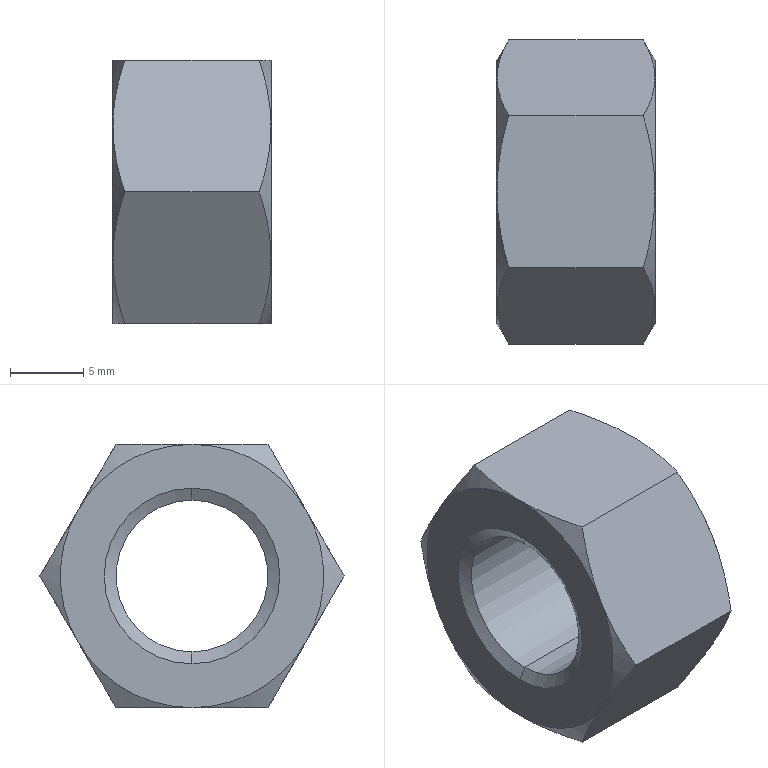Part | SolidWorks | features BaseBody 1 | 1 solid | 26 faces | box 10.8 x 20.785 x 18 mm | volume 2091 mm3 | cone 16 | plane 8 | cylinder 2 | commonest cylinder face diameters 10.376 x2
STEP:
#1=CARTESIAN_POINT('',(0.4688,0.,5.188));
#2=VERTEX_POINT('',#1);
#3=CARTESIAN_POINT('',(0.4688,0.,-5.188));
#4=VERTEX_POINT('',#3);
#5=CARTESIAN_POINT('',(0.4688,0.,0.));
#6=DIRECTION('',(1.,0.,0.));
#7=DIRECTION('',(0.,0.,-1.));
#8=AXIS2_PLACEMENT_3D('',#5,#6,#7);
#9=CIRCLE('',#8,5.188);
#10=EDGE_CURVE('',#2,#4,#9,.T.);
#11=ORIENTED_EDGE('',*,*,#10,.F.);
#12=CARTESIAN_POINT('',(10.331,0.,5.188));
#13=VERTEX_POINT('',#12);
#14=CARTESIAN_POINT('',(-18.74,0.,5.188));
#15=DIRECTION('',(1.,0.,0.));
#16=VECTOR('',#15,1000.);
#17=LINE('',#14,#16);
#18=EDGE_CURVE('',#2,#13,#17,.T.);
#19=ORIENTED_EDGE('',*,*,#18,.T.);
#20=CARTESIAN_POINT('',(10.331,0.,-5.188));
#21=VERTEX_POINT('',#20);
#22=CARTESIAN_POINT('',(10.331,0.,0.));
#23=DIRECTION('',(-1.,0.,0.));
#24=DIRECTION('',(0.,0.,-1.));
#25=AXIS2_PLACEMENT_3D('',#22,#23,#24);
#26=CIRCLE('',#25,5.188);
#27=EDGE_CURVE('',#21,#13,#26,.T.);
#28=ORIENTED_EDGE('',*,*,#27,.F.);
#29=CARTESIAN_POINT('',(-18.74,0.,-5.188));
#30=DIRECTION('',(1.,0.,0.));
#31=VECTOR('',#30,1000.);
#32=LINE('',#29,#31);
#33=EDGE_CURVE('',#4,#21,#32,.T.);
#34=ORIENTED_EDGE('',*,*,#33,.F.);
#35=EDGE_LOOP('',(#11,#19,#28,#34));
#36=FACE_OUTER_BOUND('',#35,.T.);
#37=CARTESIAN_POINT('',(-18.74,0.,0.));
#38=DIRECTION('',(1.,0.,0.));
#39=DIRECTION('',(0.,0.,-1.));
#40=AXIS2_PLACEMENT_3D('',#37,#38,#39);
#41=CYLINDRICAL_SURFACE('',#40,5.188);
#42=ADVANCED_FACE('',(#36),#41,.F.);
#43=ORIENTED_EDGE('',*,*,#10,.T.);
#44=CARTESIAN_POINT('',(0.,0.,-6.));
#45=VERTEX_POINT('',#44);
#46=CARTESIAN_POINT('',(0.,0.,-6.));
#47=DIRECTION('',(-0.5,0.,-0.866));
#48=VECTOR('',#47,1000.);
#49=LINE('',#46,#48);
#50=EDGE_CURVE('',#4,#45,#49,.T.);
#51=ORIENTED_EDGE('',*,*,#50,.T.);
#52=CARTESIAN_POINT('',(0.,0.,6.));
#53=VERTEX_POINT('',#52);
#54=CARTESIAN_POINT('',(0.,0.,0.));
#55=DIRECTION('',(1.,0.,0.));
#56=DIRECTION('',(0.,0.,1.));
#57=AXIS2_PLACEMENT_3D('',#54,#55,#56);
#58=CIRCLE('',#57,6.);
#59=EDGE_CURVE('',#53,#45,#58,.T.);
#60=ORIENTED_EDGE('',*,*,#59,.F.);
#61=CARTESIAN_POINT('',(0.,0.,6.));
#62=DIRECTION('',(-0.5,0.,0.866));
#63=VECTOR('',#62,1000.);
#64=LINE('',#61,#63);
#65=EDGE_CURVE('',#2,#53,#64,.T.);
#66=ORIENTED_EDGE('',*,*,#65,.F.);
#67=EDGE_LOOP('',(#43,#51,#60,#66));
#68=FACE_OUTER_BOUND('',#67,.T.);
#69=CARTESIAN_POINT('',(0.,0.,0.));
#70=DIRECTION('',(-1.,0.,0.));
#71=DIRECTION('',(0.,0.,1.));
#72=AXIS2_PLACEMENT_3D('',#69,#70,#71);
#73=CONICAL_SURFACE('',#72,6.,1.047);
#74=ADVANCED_FACE('',(#68),#73,.F.);
#75=ORIENTED_EDGE('',*,*,#27,.T.);
#76=CARTESIAN_POINT('',(10.8,0.,6.));
#77=VERTEX_POINT('',#76);
#78=CARTESIAN_POINT('',(10.8,0.,6.));
#79=DIRECTION('',(0.5,0.,0.866));
#80=VECTOR('',#79,1000.);
#81=LINE('',#78,#80);
#82=EDGE_CURVE('',#13,#77,#81,.T.);
#83=ORIENTED_EDGE('',*,*,#82,.T.);
#84=CARTESIAN_POINT('',(10.8,0.,-6.));
#85=VERTEX_POINT('',#84);
#86=CARTESIAN_POINT('',(10.8,0.,0.));
#87=DIRECTION('',(-1.,0.,0.));
#88=DIRECTION('',(0.,0.,-1.));
#89=AXIS2_PLACEMENT_3D('',#86,#87,#88);
#90=CIRCLE('',#89,6.);
#91=EDGE_CURVE('',#85,#77,#90,.T.);
#92=ORIENTED_EDGE('',*,*,#91,.F.);
#93=CARTESIAN_POINT('',(10.8,0.,-6.));
#94=DIRECTION('',(0.5,0.,-0.866));
#95=VECTOR('',#94,1000.);
#96=LINE('',#93,#95);
#97=EDGE_CURVE('',#21,#85,#96,.T.);
#98=ORIENTED_EDGE('',*,*,#97,.F.);
#99=EDGE_LOOP('',(#75,#83,#92,#98));
#100=FACE_OUTER_BOUND('',#99,.T.);
#101=CARTESIAN_POINT('',(10.8,0.,0.));
#102=DIRECTION('',(1.,0.,0.));
#103=DIRECTION('',(0.,0.,-1.));
#104=AXIS2_PLACEMENT_3D('',#101,#102,#103);
#105=CONICAL_SURFACE('',#104,6.,1.047);
#106=ADVANCED_FACE('',(#100),#105,.F.);
#107=ORIENTED_EDGE('',*,*,#18,.F.);
#108=CARTESIAN_POINT('',(0.4688,0.,0.));
#109=DIRECTION('',(1.,0.,0.));
#110=DIRECTION('',(0.,0.,-1.));
#111=AXIS2_PLACEMENT_3D('',#108,#109,#110);
#112=CIRCLE('',#111,5.188);
#113=EDGE_CURVE('',#4,#2,#112,.T.);
#114=ORIENTED_EDGE('',*,*,#113,.F.);
#115=ORIENTED_EDGE('',*,*,#33,.T.);
#116=CARTESIAN_POINT('',(10.331,0.,0.));
#117=DIRECTION('',(-1.,0.,0.));
#118=DIRECTION('',(0.,0.,-1.));
#119=AXIS2_PLACEMENT_3D('',#116,#117,#118);
#120=CIRCLE('',#119,5.188);
#121=EDGE_CURVE('',#13,#21,#120,.T.);
#122=ORIENTED_EDGE('',*,*,#121,.F.);
#123=EDGE_LOOP('',(#107,#114,#115,#122));
#124=FACE_OUTER_BOUND('',#123,.T.);
#125=CARTESIAN_POINT('',(-18.74,0.,0.));
#126=DIRECTION('',(1.,0.,0.));
#127=DIRECTION('',(0.,0.,-1.));
#128=AXIS2_PLACEMENT_3D('',#125,#126,#127);
#129=CYLINDRICAL_SURFACE('',#128,5.188);
#130=ADVANCED_FACE('',(#124),#129,.F.);
#131=ORIENTED_EDGE('',*,*,#50,.F.);
#132=ORIENTED_EDGE('',*,*,#113,.T.);
#133=ORIENTED_EDGE('',*,*,#65,.T.);
#134=CARTESIAN_POINT('',(0.,0.,0.));
#135=DIRECTION('',(1.,0.,0.));
#136=DIRECTION('',(0.,0.,1.));
#137=AXIS2_PLACEMENT_3D('',#134,#135,#136);
#138=CIRCLE('',#137,6.);
#139=EDGE_CURVE('',#45,#53,#138,.T.);
#140=ORIENTED_EDGE('',*,*,#139,.F.);
#141=EDGE_LOOP('',(#131,#132,#133,#140));
#142=FACE_OUTER_BOUND('',#141,.T.);
#143=CARTESIAN_POINT('',(0.,0.,0.));
#144=DIRECTION('',(-1.,0.,0.));
#145=DIRECTION('',(0.,0.,1.));
#146=AXIS2_PLACEMENT_3D('',#143,#144,#145);
#147=CONICAL_SURFACE('',#146,6.,1.047);
#148=ADVANCED_FACE('',(#142),#147,.F.);
#149=ORIENTED_EDGE('',*,*,#82,.F.);
#150=ORIENTED_EDGE('',*,*,#121,.T.);
#151=ORIENTED_EDGE('',*,*,#97,.T.);
#152=CARTESIAN_POINT('',(10.8,0.,0.));
#153=DIRECTION('',(-1.,0.,0.));
#154=DIRECTION('',(0.,0.,-1.));
#155=AXIS2_PLACEMENT_3D('',#152,#153,#154);
#156=CIRCLE('',#155,6.);
#157=EDGE_CURVE('',#77,#85,#156,.T.);
#158=ORIENTED_EDGE('',*,*,#157,.F.);
#159=EDGE_LOOP('',(#149,#150,#151,#158));
#160=FACE_OUTER_BOUND('',#159,.T.);
#161=CARTESIAN_POINT('',(10.8,0.,0.));
#162=DIRECTION('',(1.,0.,0.));
#163=DIRECTION('',(0.,0.,-1.));
#164=AXIS2_PLACEMENT_3D('',#161,#162,#163);
#165=CONICAL_SURFACE('',#164,6.,1.047);
#166=ADVANCED_FACE('',(#160),#165,.F.);
#167=ORIENTED_EDGE('',*,*,#59,.T.);
#168=ORIENTED_EDGE('',*,*,#139,.T.);
#169=EDGE_LOOP('',(#167,#168));
#170=FACE_BOUND('',#169,.T.);
#171=CARTESIAN_POINT('',(0.,0.,9.));
#172=VERTEX_POINT('',#171);
#173=CARTESIAN_POINT('',(0.,-7.794,4.5));
#174=VERTEX_POINT('',#173);
#175=CARTESIAN_POINT('',(0.,0.,0.));
#176=DIRECTION('',(1.,0.,0.));
#177=DIRECTION('',(0.,0.,-1.));
#178=AXIS2_PLACEMENT_3D('',#175,#176,#177);
#179=CIRCLE('',#178,9.);
#180=EDGE_CURVE('',#172,#174,#179,.T.);
#181=ORIENTED_EDGE('',*,*,#180,.F.);
#182=CARTESIAN_POINT('',(0.,7.794,4.5));
#183=VERTEX_POINT('',#182);
#184=CARTESIAN_POINT('',(0.,0.,0.));
#185=DIRECTION('',(1.,0.,0.));
#186=DIRECTION('',(0.,0.,-1.));
#187=AXIS2_PLACEMENT_3D('',#184,#185,#186);
#188=CIRCLE('',#187,9.);
#189=EDGE_CURVE('',#183,#172,#188,.T.);
#190=ORIENTED_EDGE('',*,*,#189,.F.);
#191=CARTESIAN_POINT('',(0.,7.794,-4.5));
#192=VERTEX_POINT('',#191);
#193=CARTESIAN_POINT('',(0.,0.,0.));
#194=DIRECTION('',(1.,0.,0.));
#195=DIRECTION('',(0.,0.,-1.));
#196=AXIS2_PLACEMENT_3D('',#193,#194,#195);
#197=CIRCLE('',#196,9.);
#198=EDGE_CURVE('',#192,#183,#197,.T.);
#199=ORIENTED_EDGE('',*,*,#198,.F.);
#200=CARTESIAN_POINT('',(0.,0.,-9.));
#201=VERTEX_POINT('',#200);
#202=CARTESIAN_POINT('',(0.,0.,0.));
#203=DIRECTION('',(1.,0.,0.));
#204=DIRECTION('',(0.,0.,-1.));
#205=AXIS2_PLACEMENT_3D('',#202,#203,#204);
#206=CIRCLE('',#205,9.);
#207=EDGE_CURVE('',#201,#192,#206,.T.);
#208=ORIENTED_EDGE('',*,*,#207,.F.);
#209=CARTESIAN_POINT('',(0.,-7.794,-4.5));
#210=VERTEX_POINT('',#209);
#211=CARTESIAN_POINT('',(0.,0.,0.));
#212=DIRECTION('',(1.,0.,0.));
#213=DIRECTION('',(0.,0.,-1.));
#214=AXIS2_PLACEMENT_3D('',#211,#212,#213);
#215=CIRCLE('',#214,9.);
#216=EDGE_CURVE('',#210,#201,#215,.T.);
#217=ORIENTED_EDGE('',*,*,#216,.F.);
#218=CARTESIAN_POINT('',(0.,0.,0.));
#219=DIRECTION('',(1.,0.,0.));
#220=DIRECTION('',(0.,0.,-1.));
#221=AXIS2_PLACEMENT_3D('',#218,#219,#220);
#222=CIRCLE('',#221,9.);
#223=EDGE_CURVE('',#174,#210,#222,.T.);
#224=ORIENTED_EDGE('',*,*,#223,.F.);
#225=EDGE_LOOP('',(#181,#190,#199,#208,#217,#224));
#226=FACE_OUTER_BOUND('',#225,.T.);
#227=CARTESIAN_POINT('',(0.,0.,0.));
#228=DIRECTION('',(1.,0.,0.));
#229=DIRECTION('',(0.,0.,-1.));
#230=AXIS2_PLACEMENT_3D('',#227,#228,#229);
#231=PLANE('',#230);
#232=ADVANCED_FACE('',(#170,#226),#231,.F.);
#233=ORIENTED_EDGE('',*,*,#91,.T.);
#234=ORIENTED_EDGE('',*,*,#157,.T.);
#235=EDGE_LOOP('',(#233,#234));
#236=FACE_BOUND('',#235,.T.);
#237=CARTESIAN_POINT('',(10.8,0.,9.));
#238=VERTEX_POINT('',#237);
#239=CARTESIAN_POINT('',(10.8,-7.794,4.5));
#240=VERTEX_POINT('',#239);
#241=CARTESIAN_POINT('',(10.8,0.,0.));
#242=DIRECTION('',(1.,0.,0.));
#243=DIRECTION('',(0.,0.,1.));
#244=AXIS2_PLACEMENT_3D('',#241,#242,#243);
#245=CIRCLE('',#244,9.);
#246=EDGE_CURVE('',#238,#240,#245,.T.);
#247=ORIENTED_EDGE('',*,*,#246,.T.);
#248=CARTESIAN_POINT('',(10.8,-7.794,-4.5));
#249=VERTEX_POINT('',#248);
#250=CARTESIAN_POINT('',(10.8,0.,0.));
#251=DIRECTION('',(1.,0.,0.));
#252=DIRECTION('',(0.,0.,1.));
#253=AXIS2_PLACEMENT_3D('',#250,#251,#252);
#254=CIRCLE('',#253,9.);
#255=EDGE_CURVE('',#240,#249,#254,.T.);
#256=ORIENTED_EDGE('',*,*,#255,.T.);
#257=CARTESIAN_POINT('',(10.8,0.,-9.));
#258=VERTEX_POINT('',#257);
#259=CARTESIAN_POINT('',(10.8,0.,0.));
#260=DIRECTION('',(1.,0.,0.));
#261=DIRECTION('',(0.,0.,1.));
#262=AXIS2_PLACEMENT_3D('',#259,#260,#261);
#263=CIRCLE('',#262,9.);
#264=EDGE_CURVE('',#249,#258,#263,.T.);
#265=ORIENTED_EDGE('',*,*,#264,.T.);
#266=CARTESIAN_POINT('',(10.8,7.794,-4.5));
#267=VERTEX_POINT('',#266);
#268=CARTESIAN_POINT('',(10.8,0.,0.));
#269=DIRECTION('',(1.,0.,0.));
#270=DIRECTION('',(0.,0.,1.));
#271=AXIS2_PLACEMENT_3D('',#268,#269,#270);
#272=CIRCLE('',#271,9.);
#273=EDGE_CURVE('',#258,#267,#272,.T.);
#274=ORIENTED_EDGE('',*,*,#273,.T.);
#275=CARTESIAN_POINT('',(10.8,7.794,4.5));
#276=VERTEX_POINT('',#275);
#277=CARTESIAN_POINT('',(10.8,0.,0.));
#278=DIRECTION('',(1.,0.,0.));
#279=DIRECTION('',(0.,0.,1.));
#280=AXIS2_PLACEMENT_3D('',#277,#278,#279);
#281=CIRCLE('',#280,9.);
#282=EDGE_CURVE('',#267,#276,#281,.T.);
#283=ORIENTED_EDGE('',*,*,#282,.T.);
#284=CARTESIAN_POINT('',(10.8,0.,0.));
#285=DIRECTION('',(1.,0.,0.));
#286=DIRECTION('',(0.,0.,1.));
#287=AXIS2_PLACEMENT_3D('',#284,#285,#286);
#288=CIRCLE('',#287,9.);
#289=EDGE_CURVE('',#276,#238,#288,.T.);
#290=ORIENTED_EDGE('',*,*,#289,.T.);
#291=EDGE_LOOP('',(#247,#256,#265,#274,#283,#290));
#292=FACE_OUTER_BOUND('',#291,.T.);
#293=CARTESIAN_POINT('',(10.8,0.,0.));
#294=DIRECTION('',(1.,0.,0.));
#295=DIRECTION('',(0.,0.,-1.));
#296=AXIS2_PLACEMENT_3D('',#293,#294,#295);
#297=PLANE('',#296);
#298=ADVANCED_FACE('',(#236,#292),#297,.T.);
#299=ORIENTED_EDGE('',*,*,#223,.T.);
#300=CARTESIAN_POINT('',(0.8038,-10.392,0.000000014));
#301=VERTEX_POINT('',#300);
#302=CARTESIAN_POINT('',(0.,-7.794,-4.5));
#303=CARTESIAN_POINT('',(0.,-8.238,-3.732));
#304=CARTESIAN_POINT('',(0.07685,-8.675,-2.974));
#305=CARTESIAN_POINT('',(0.3567,-9.54,-1.476));
#306=CARTESIAN_POINT('',(0.5588,-9.968,-0.7351));
#307=CARTESIAN_POINT('',(0.8038,-10.392,0.000000014));
#308=B_SPLINE_CURVE_WITH_KNOTS('',3,(#302,#303,#304,#305,#306,#307),.UNSPECIFIED.,.F.,.F.,(4,2,4),(0.,0.002629,0.005258),.UNSPECIFIED.);
#309=EDGE_CURVE('',#210,#301,#308,.T.);
#310=ORIENTED_EDGE('',*,*,#309,.T.);
#311=CARTESIAN_POINT('',(0.8038,-10.392,0.000000014));
#312=CARTESIAN_POINT('',(0.5588,-9.968,0.7351));
#313=CARTESIAN_POINT('',(0.3567,-9.54,1.476));
#314=CARTESIAN_POINT('',(0.07685,-8.675,2.974));
#315=CARTESIAN_POINT('',(0.,-8.238,3.732));
#316=CARTESIAN_POINT('',(0.,-7.794,4.5));
#317=B_SPLINE_CURVE_WITH_KNOTS('',3,(#311,#312,#313,#314,#315,#316),.UNSPECIFIED.,.F.,.F.,(4,2,4),(0.,0.002629,0.005258),.UNSPECIFIED.);
#318=EDGE_CURVE('',#301,#174,#317,.T.);
#319=ORIENTED_EDGE('',*,*,#318,.T.);
#320=EDGE_LOOP('',(#299,#310,#319));
#321=FACE_OUTER_BOUND('',#320,.T.);
#322=CARTESIAN_POINT('',(0.8087,0.,0.));
#323=DIRECTION('',(1.,0.,0.));
#324=DIRECTION('',(0.,0.,-1.));
#325=AXIS2_PLACEMENT_3D('',#322,#323,#324);
#326=CONICAL_SURFACE('',#325,10.401,1.047);
#327=ADVANCED_FACE('',(#321),#326,.T.);
#328=ORIENTED_EDGE('',*,*,#180,.T.);
#329=CARTESIAN_POINT('',(0.8038,-5.196,9.));
#330=VERTEX_POINT('',#329);
#331=CARTESIAN_POINT('',(0.,-7.794,4.5));
#332=CARTESIAN_POINT('',(0.,-7.351,5.268));
#333=CARTESIAN_POINT('',(0.07685,-6.913,6.026));
#334=CARTESIAN_POINT('',(0.3567,-6.048,7.524));
#335=CARTESIAN_POINT('',(0.5588,-5.621,8.265));
#336=CARTESIAN_POINT('',(0.8038,-5.196,9.));
#337=B_SPLINE_CURVE_WITH_KNOTS('',3,(#331,#332,#333,#334,#335,#336),.UNSPECIFIED.,.F.,.F.,(4,2,4),(0.,0.002629,0.005258),.UNSPECIFIED.);
#338=EDGE_CURVE('',#174,#330,#337,.T.);
#339=ORIENTED_EDGE('',*,*,#338,.T.);
#340=CARTESIAN_POINT('',(0.8038,-5.196,9.));
#341=CARTESIAN_POINT('',(0.5588,-4.347,9.));
#342=CARTESIAN_POINT('',(0.3567,-3.492,9.));
#343=CARTESIAN_POINT('',(0.07685,-1.762,9.));
#344=CARTESIAN_POINT('',(0.,-0.8868,9.));
#345=CARTESIAN_POINT('',(0.,0.,9.));
#346=B_SPLINE_CURVE_WITH_KNOTS('',3,(#340,#341,#342,#343,#344,#345),.UNSPECIFIED.,.F.,.F.,(4,2,4),(0.,0.002629,0.005258),.UNSPECIFIED.);
#347=EDGE_CURVE('',#330,#172,#346,.T.);
#348=ORIENTED_EDGE('',*,*,#347,.T.);
#349=EDGE_LOOP('',(#328,#339,#348));
#350=FACE_OUTER_BOUND('',#349,.T.);
#351=CARTESIAN_POINT('',(0.8087,0.,0.));
#352=DIRECTION('',(1.,0.,0.));
#353=DIRECTION('',(0.,0.,-1.));
#354=AXIS2_PLACEMENT_3D('',#351,#352,#353);
#355=CONICAL_SURFACE('',#354,10.401,1.047);
#356=ADVANCED_FACE('',(#350),#355,.T.);
#357=ORIENTED_EDGE('',*,*,#189,.T.);
#358=CARTESIAN_POINT('',(0.8038,5.196,9.));
#359=VERTEX_POINT('',#358);
#360=CARTESIAN_POINT('',(0.,0.,9.));
#361=CARTESIAN_POINT('',(0.,0.8868,9.));
#362=CARTESIAN_POINT('',(0.07685,1.762,9.));
#363=CARTESIAN_POINT('',(0.3567,3.492,9.));
#364=CARTESIAN_POINT('',(0.5588,4.347,9.));
#365=CARTESIAN_POINT('',(0.8038,5.196,9.));
#366=B_SPLINE_CURVE_WITH_KNOTS('',3,(#360,#361,#362,#363,#364,#365),.UNSPECIFIED.,.F.,.F.,(4,2,4),(0.,0.002629,0.005258),.UNSPECIFIED.);
#367=EDGE_CURVE('',#172,#359,#366,.T.);
#368=ORIENTED_EDGE('',*,*,#367,.T.);
#369=CARTESIAN_POINT('',(0.8038,5.196,9.));
#370=CARTESIAN_POINT('',(0.5588,5.621,8.265));
#371=CARTESIAN_POINT('',(0.3567,6.048,7.524));
#372=CARTESIAN_POINT('',(0.07685,6.913,6.026));
#373=CARTESIAN_POINT('',(0.,7.351,5.268));
#374=CARTESIAN_POINT('',(0.,7.794,4.5));
#375=B_SPLINE_CURVE_WITH_KNOTS('',3,(#369,#370,#371,#372,#373,#374),.UNSPECIFIED.,.F.,.F.,(4,2,4),(0.,0.002629,0.005258),.UNSPECIFIED.);
#376=EDGE_CURVE('',#359,#183,#375,.T.);
#377=ORIENTED_EDGE('',*,*,#376,.T.);
#378=EDGE_LOOP('',(#357,#368,#377));
#379=FACE_OUTER_BOUND('',#378,.T.);
#380=CARTESIAN_POINT('',(0.8087,0.,0.));
#381=DIRECTION('',(1.,0.,0.));
#382=DIRECTION('',(0.,0.,-1.));
#383=AXIS2_PLACEMENT_3D('',#380,#381,#382);
#384=CONICAL_SURFACE('',#383,10.401,1.047);
#385=ADVANCED_FACE('',(#379),#384,.T.);
#386=ORIENTED_EDGE('',*,*,#198,.T.);
#387=CARTESIAN_POINT('',(0.8038,10.392,-0.000000014));
#388=VERTEX_POINT('',#387);
#389=CARTESIAN_POINT('',(0.,7.794,4.5));
#390=CARTESIAN_POINT('',(0.,8.238,3.732));
#391=CARTESIAN_POINT('',(0.07685,8.675,2.974));
#392=CARTESIAN_POINT('',(0.3567,9.54,1.476));
#393=CARTESIAN_POINT('',(0.5588,9.968,0.7351));
#394=CARTESIAN_POINT('',(0.8038,10.392,-0.000000014));
#395=B_SPLINE_CURVE_WITH_KNOTS('',3,(#389,#390,#391,#392,#393,#394),.UNSPECIFIED.,.F.,.F.,(4,2,4),(0.,0.002629,0.005258),.UNSPECIFIED.);
#396=EDGE_CURVE('',#183,#388,#395,.T.);
#397=ORIENTED_EDGE('',*,*,#396,.T.);
#398=CARTESIAN_POINT('',(0.8038,10.392,-0.000000014));
#399=CARTESIAN_POINT('',(0.5588,9.968,-0.7351));
#400=CARTESIAN_POINT('',(0.3567,9.54,-1.476));
#401=CARTESIAN_POINT('',(0.07685,8.675,-2.974));
#402=CARTESIAN_POINT('',(0.,8.238,-3.732));
#403=CARTESIAN_POINT('',(0.,7.794,-4.5));
#404=B_SPLINE_CURVE_WITH_KNOTS('',3,(#398,#399,#400,#401,#402,#403),.UNSPECIFIED.,.F.,.F.,(4,2,4),(0.,0.002629,0.005258),.UNSPECIFIED.);
#405=EDGE_CURVE('',#388,#192,#404,.T.);
#406=ORIENTED_EDGE('',*,*,#405,.T.);
#407=EDGE_LOOP('',(#386,#397,#406));
#408=FACE_OUTER_BOUND('',#407,.T.);
#409=CARTESIAN_POINT('',(0.8087,0.,0.));
#410=DIRECTION('',(1.,0.,0.));
#411=DIRECTION('',(0.,0.,-1.));
#412=AXIS2_PLACEMENT_3D('',#409,#410,#411);
#413=CONICAL_SURFACE('',#412,10.401,1.047);
#414=ADVANCED_FACE('',(#408),#413,.T.);
#415=CARTESIAN_POINT('',(0.8038,5.196,-9.));
#416=VERTEX_POINT('',#415);
#417=CARTESIAN_POINT('',(0.8038,5.196,-9.));
#418=CARTESIAN_POINT('',(0.5588,4.347,-9.));
#419=CARTESIAN_POINT('',(0.3567,3.492,-9.));
#420=CARTESIAN_POINT('',(0.07685,1.762,-9.));
#421=CARTESIAN_POINT('',(0.,0.8868,-9.));
#422=CARTESIAN_POINT('',(0.,0.,-9.));
#423=B_SPLINE_CURVE_WITH_KNOTS('',3,(#417,#418,#419,#420,#421,#422),.UNSPECIFIED.,.F.,.F.,(4,2,4),(0.,0.002629,0.005258),.UNSPECIFIED.);
#424=EDGE_CURVE('',#416,#201,#423,.T.);
#425=ORIENTED_EDGE('',*,*,#424,.T.);
#426=ORIENTED_EDGE('',*,*,#207,.T.);
#427=CARTESIAN_POINT('',(0.,7.794,-4.5));
#428=CARTESIAN_POINT('',(0.,7.351,-5.268));
#429=CARTESIAN_POINT('',(0.07685,6.913,-6.026));
#430=CARTESIAN_POINT('',(0.3567,6.048,-7.524));
#431=CARTESIAN_POINT('',(0.5588,5.621,-8.265));
#432=CARTESIAN_POINT('',(0.8038,5.196,-9.));
#433=B_SPLINE_CURVE_WITH_KNOTS('',3,(#427,#428,#429,#430,#431,#432),.UNSPECIFIED.,.F.,.F.,(4,2,4),(0.,0.002629,0.005258),.UNSPECIFIED.);
#434=EDGE_CURVE('',#192,#416,#433,.T.);
#435=ORIENTED_EDGE('',*,*,#434,.T.);
#436=EDGE_LOOP('',(#425,#426,#435));
#437=FACE_OUTER_BOUND('',#436,.T.);
#438=CARTESIAN_POINT('',(0.8087,0.,0.));
#439=DIRECTION('',(1.,0.,0.));
#440=DIRECTION('',(0.,0.,-1.));
#441=AXIS2_PLACEMENT_3D('',#438,#439,#440);
#442=CONICAL_SURFACE('',#441,10.401,1.047);
#443=ADVANCED_FACE('',(#437),#442,.T.);
#444=CARTESIAN_POINT('',(0.8038,-5.196,-9.));
#445=VERTEX_POINT('',#444);
#446=CARTESIAN_POINT('',(0.8038,-5.196,-9.));
#447=CARTESIAN_POINT('',(0.5588,-5.621,-8.265));
#448=CARTESIAN_POINT('',(0.3567,-6.048,-7.524));
#449=CARTESIAN_POINT('',(0.07685,-6.913,-6.026));
#450=CARTESIAN_POINT('',(0.,-7.351,-5.268));
#451=CARTESIAN_POINT('',(0.,-7.794,-4.5));
#452=B_SPLINE_CURVE_WITH_KNOTS('',3,(#446,#447,#448,#449,#450,#451),.UNSPECIFIED.,.F.,.F.,(4,2,4),(0.,0.002629,0.005258),.UNSPECIFIED.);
#453=EDGE_CURVE('',#445,#210,#452,.T.);
#454=ORIENTED_EDGE('',*,*,#453,.T.);
#455=ORIENTED_EDGE('',*,*,#216,.T.);
#456=CARTESIAN_POINT('',(0.,0.,-9.));
#457=CARTESIAN_POINT('',(0.,-0.8868,-9.));
#458=CARTESIAN_POINT('',(0.07685,-1.762,-9.));
#459=CARTESIAN_POINT('',(0.3567,-3.492,-9.));
#460=CARTESIAN_POINT('',(0.5588,-4.347,-9.));
#461=CARTESIAN_POINT('',(0.8038,-5.196,-9.));
#462=B_SPLINE_CURVE_WITH_KNOTS('',3,(#456,#457,#458,#459,#460,#461),.UNSPECIFIED.,.F.,.F.,(4,2,4),(0.,0.002629,0.005258),.UNSPECIFIED.);
#463=EDGE_CURVE('',#201,#445,#462,.T.);
#464=ORIENTED_EDGE('',*,*,#463,.T.);
#465=EDGE_LOOP('',(#454,#455,#464));
#466=FACE_OUTER_BOUND('',#465,.T.);
#467=CARTESIAN_POINT('',(0.8087,0.,0.));
#468=DIRECTION('',(1.,0.,0.));
#469=DIRECTION('',(0.,0.,-1.));
#470=AXIS2_PLACEMENT_3D('',#467,#468,#469);
#471=CONICAL_SURFACE('',#470,10.401,1.047);
#472=ADVANCED_FACE('',(#466),#471,.T.);
#473=CARTESIAN_POINT('',(9.996,-10.392,0.000000038));
#474=VERTEX_POINT('',#473);
#475=CARTESIAN_POINT('',(9.996,-10.392,0.000000038));
#476=CARTESIAN_POINT('',(10.241,-9.968,-0.7351));
#477=CARTESIAN_POINT('',(10.443,-9.54,-1.476));
#478=CARTESIAN_POINT('',(10.723,-8.675,-2.974));
#479=CARTESIAN_POINT('',(10.8,-8.238,-3.732));
#480=CARTESIAN_POINT('',(10.8,-7.794,-4.5));
#481=B_SPLINE_CURVE_WITH_KNOTS('',3,(#475,#476,#477,#478,#479,#480),.UNSPECIFIED.,.F.,.F.,(4,2,4),(0.,0.002629,0.005258),.UNSPECIFIED.);
#482=EDGE_CURVE('',#474,#249,#481,.T.);
#483=ORIENTED_EDGE('',*,*,#482,.T.);
#484=ORIENTED_EDGE('',*,*,#255,.F.);
#485=CARTESIAN_POINT('',(10.8,-7.794,4.5));
#486=CARTESIAN_POINT('',(10.8,-8.238,3.732));
#487=CARTESIAN_POINT('',(10.723,-8.675,2.974));
#488=CARTESIAN_POINT('',(10.443,-9.54,1.476));
#489=CARTESIAN_POINT('',(10.241,-9.968,0.7351));
#490=CARTESIAN_POINT('',(9.996,-10.392,0.000000038));
#491=B_SPLINE_CURVE_WITH_KNOTS('',3,(#485,#486,#487,#488,#489,#490),.UNSPECIFIED.,.F.,.F.,(4,2,4),(0.,0.002629,0.005258),.UNSPECIFIED.);
#492=EDGE_CURVE('',#240,#474,#491,.T.);
#493=ORIENTED_EDGE('',*,*,#492,.T.);
#494=EDGE_LOOP('',(#483,#484,#493));
#495=FACE_OUTER_BOUND('',#494,.T.);
#496=CARTESIAN_POINT('',(9.991,0.,0.));
#497=DIRECTION('',(-1.,0.,0.));
#498=DIRECTION('',(0.,0.,1.));
#499=AXIS2_PLACEMENT_3D('',#496,#497,#498);
#500=CONICAL_SURFACE('',#499,10.401,1.047);
#501=ADVANCED_FACE('',(#495),#500,.T.);
#502=CARTESIAN_POINT('',(9.996,-5.196,9.));
#503=VERTEX_POINT('',#502);
#504=CARTESIAN_POINT('',(9.996,-5.196,9.));
#505=CARTESIAN_POINT('',(10.241,-5.621,8.265));
#506=CARTESIAN_POINT('',(10.443,-6.048,7.524));
#507=CARTESIAN_POINT('',(10.723,-6.913,6.026));
#508=CARTESIAN_POINT('',(10.8,-7.351,5.268));
#509=CARTESIAN_POINT('',(10.8,-7.794,4.5));
#510=B_SPLINE_CURVE_WITH_KNOTS('',3,(#504,#505,#506,#507,#508,#509),.UNSPECIFIED.,.F.,.F.,(4,2,4),(0.,0.002629,0.005258),.UNSPECIFIED.);
#511=EDGE_CURVE('',#503,#240,#510,.T.);
#512=ORIENTED_EDGE('',*,*,#511,.T.);
#513=ORIENTED_EDGE('',*,*,#246,.F.);
#514=CARTESIAN_POINT('',(10.8,0.,9.));
#515=CARTESIAN_POINT('',(10.8,-0.8868,9.));
#516=CARTESIAN_POINT('',(10.723,-1.762,9.));
#517=CARTESIAN_POINT('',(10.443,-3.492,9.));
#518=CARTESIAN_POINT('',(10.241,-4.347,9.));
#519=CARTESIAN_POINT('',(9.996,-5.196,9.));
#520=B_SPLINE_CURVE_WITH_KNOTS('',3,(#514,#515,#516,#517,#518,#519),.UNSPECIFIED.,.F.,.F.,(4,2,4),(0.,0.002629,0.005258),.UNSPECIFIED.);
#521=EDGE_CURVE('',#238,#503,#520,.T.);
#522=ORIENTED_EDGE('',*,*,#521,.T.);
#523=EDGE_LOOP('',(#512,#513,#522));
#524=FACE_OUTER_BOUND('',#523,.T.);
#525=CARTESIAN_POINT('',(9.991,0.,0.));
#526=DIRECTION('',(-1.,0.,0.));
#527=DIRECTION('',(0.,0.,1.));
#528=AXIS2_PLACEMENT_3D('',#525,#526,#527);
#529=CONICAL_SURFACE('',#528,10.401,1.047);
#530=ADVANCED_FACE('',(#524),#529,.T.);
#531=CARTESIAN_POINT('',(9.996,5.196,9.));
#532=VERTEX_POINT('',#531);
#533=CARTESIAN_POINT('',(9.996,5.196,9.));
#534=CARTESIAN_POINT('',(10.241,4.347,9.));
#535=CARTESIAN_POINT('',(10.443,3.492,9.));
#536=CARTESIAN_POINT('',(10.723,1.762,9.));
#537=CARTESIAN_POINT('',(10.8,0.8868,9.));
#538=CARTESIAN_POINT('',(10.8,0.,9.));
#539=B_SPLINE_CURVE_WITH_KNOTS('',3,(#533,#534,#535,#536,#537,#538),.UNSPECIFIED.,.F.,.F.,(4,2,4),(0.,0.002629,0.005258),.UNSPECIFIED.);
#540=EDGE_CURVE('',#532,#238,#539,.T.);
#541=ORIENTED_EDGE('',*,*,#540,.T.);
#542=ORIENTED_EDGE('',*,*,#289,.F.);
#543=CARTESIAN_POINT('',(10.8,7.794,4.5));
#544=CARTESIAN_POINT('',(10.8,7.351,5.268));
#545=CARTESIAN_POINT('',(10.723,6.913,6.026));
#546=CARTESIAN_POINT('',(10.443,6.048,7.524));
#547=CARTESIAN_POINT('',(10.241,5.621,8.265));
#548=CARTESIAN_POINT('',(9.996,5.196,9.));
#549=B_SPLINE_CURVE_WITH_KNOTS('',3,(#543,#544,#545,#546,#547,#548),.UNSPECIFIED.,.F.,.F.,(4,2,4),(0.,0.002629,0.005258),.UNSPECIFIED.);
#550=EDGE_CURVE('',#276,#532,#549,.T.);
#551=ORIENTED_EDGE('',*,*,#550,.T.);
#552=EDGE_LOOP('',(#541,#542,#551));
#553=FACE_OUTER_BOUND('',#552,.T.);
#554=CARTESIAN_POINT('',(9.991,0.,0.));
#555=DIRECTION('',(-1.,0.,0.));
#556=DIRECTION('',(0.,0.,1.));
#557=AXIS2_PLACEMENT_3D('',#554,#555,#556);
#558=CONICAL_SURFACE('',#557,10.401,1.047);
#559=ADVANCED_FACE('',(#553),#558,.T.);
#560=ORIENTED_EDGE('',*,*,#282,.F.);
#561=CARTESIAN_POINT('',(9.996,10.392,0.000000014));
#562=VERTEX_POINT('',#561);
#563=CARTESIAN_POINT('',(10.8,7.794,-4.5));
#564=CARTESIAN_POINT('',(10.8,8.238,-3.732));
#565=CARTESIAN_POINT('',(10.723,8.675,-2.974));
#566=CARTESIAN_POINT('',(10.443,9.54,-1.476));
#567=CARTESIAN_POINT('',(10.241,9.968,-0.7351));
#568=CARTESIAN_POINT('',(9.996,10.392,0.000000014));
#569=B_SPLINE_CURVE_WITH_KNOTS('',3,(#563,#564,#565,#566,#567,#568),.UNSPECIFIED.,.F.,.F.,(4,2,4),(0.,0.002629,0.005258),.UNSPECIFIED.);
#570=EDGE_CURVE('',#267,#562,#569,.T.);
#571=ORIENTED_EDGE('',*,*,#570,.T.);
#572=CARTESIAN_POINT('',(9.996,10.392,0.000000014));
#573=CARTESIAN_POINT('',(10.241,9.968,0.7351));
#574=CARTESIAN_POINT('',(10.443,9.54,1.476));
#575=CARTESIAN_POINT('',(10.723,8.675,2.974));
#576=CARTESIAN_POINT('',(10.8,8.238,3.732));
#577=CARTESIAN_POINT('',(10.8,7.794,4.5));
#578=B_SPLINE_CURVE_WITH_KNOTS('',3,(#572,#573,#574,#575,#576,#577),.UNSPECIFIED.,.F.,.F.,(4,2,4),(0.,0.002629,0.005258),.UNSPECIFIED.);
#579=EDGE_CURVE('',#562,#276,#578,.T.);
#580=ORIENTED_EDGE('',*,*,#579,.T.);
#581=EDGE_LOOP('',(#560,#571,#580));
#582=FACE_OUTER_BOUND('',#581,.T.);
#583=CARTESIAN_POINT('',(9.991,0.,0.));
#584=DIRECTION('',(-1.,0.,0.));
#585=DIRECTION('',(0.,0.,1.));
#586=AXIS2_PLACEMENT_3D('',#583,#584,#585);
#587=CONICAL_SURFACE('',#586,10.401,1.047);
#588=ADVANCED_FACE('',(#582),#587,.T.);
#589=ORIENTED_EDGE('',*,*,#273,.F.);
#590=CARTESIAN_POINT('',(9.996,5.196,-9.));
#591=VERTEX_POINT('',#590);
#592=CARTESIAN_POINT('',(10.8,0.,-9.));
#593=CARTESIAN_POINT('',(10.8,0.8868,-9.));
#594=CARTESIAN_POINT('',(10.723,1.762,-9.));
#595=CARTESIAN_POINT('',(10.443,3.492,-9.));
#596=CARTESIAN_POINT('',(10.241,4.347,-9.));
#597=CARTESIAN_POINT('',(9.996,5.196,-9.));
#598=B_SPLINE_CURVE_WITH_KNOTS('',3,(#592,#593,#594,#595,#596,#597),.UNSPECIFIED.,.F.,.F.,(4,2,4),(0.,0.002629,0.005258),.UNSPECIFIED.);
#599=EDGE_CURVE('',#258,#591,#598,.T.);
#600=ORIENTED_EDGE('',*,*,#599,.T.);
#601=CARTESIAN_POINT('',(9.996,5.196,-9.));
#602=CARTESIAN_POINT('',(10.241,5.621,-8.265));
#603=CARTESIAN_POINT('',(10.443,6.048,-7.524));
#604=CARTESIAN_POINT('',(10.723,6.913,-6.026));
#605=CARTESIAN_POINT('',(10.8,7.351,-5.268));
#606=CARTESIAN_POINT('',(10.8,7.794,-4.5));
#607=B_SPLINE_CURVE_WITH_KNOTS('',3,(#601,#602,#603,#604,#605,#606),.UNSPECIFIED.,.F.,.F.,(4,2,4),(0.,0.002629,0.005258),.UNSPECIFIED.);
#608=EDGE_CURVE('',#591,#267,#607,.T.);
#609=ORIENTED_EDGE('',*,*,#608,.T.);
#610=EDGE_LOOP('',(#589,#600,#609));
#611=FACE_OUTER_BOUND('',#610,.T.);
#612=CARTESIAN_POINT('',(9.991,0.,0.));
#613=DIRECTION('',(-1.,0.,0.));
#614=DIRECTION('',(0.,0.,1.));
#615=AXIS2_PLACEMENT_3D('',#612,#613,#614);
#616=CONICAL_SURFACE('',#615,10.401,1.047);
#617=ADVANCED_FACE('',(#611),#616,.T.);
#618=ORIENTED_EDGE('',*,*,#264,.F.);
#619=CARTESIAN_POINT('',(9.996,-5.196,-9.));
#620=VERTEX_POINT('',#619);
#621=CARTESIAN_POINT('',(10.8,-7.794,-4.5));
#622=CARTESIAN_POINT('',(10.8,-7.351,-5.268));
#623=CARTESIAN_POINT('',(10.723,-6.913,-6.026));
#624=CARTESIAN_POINT('',(10.443,-6.048,-7.524));
#625=CARTESIAN_POINT('',(10.241,-5.621,-8.265));
#626=CARTESIAN_POINT('',(9.996,-5.196,-9.));
#627=B_SPLINE_CURVE_WITH_KNOTS('',3,(#621,#622,#623,#624,#625,#626),.UNSPECIFIED.,.F.,.F.,(4,2,4),(0.,0.002629,0.005258),.UNSPECIFIED.);
#628=EDGE_CURVE('',#249,#620,#627,.T.);
#629=ORIENTED_EDGE('',*,*,#628,.T.);
#630=CARTESIAN_POINT('',(9.996,-5.196,-9.));
#631=CARTESIAN_POINT('',(10.241,-4.347,-9.));
#632=CARTESIAN_POINT('',(10.443,-3.492,-9.));
#633=CARTESIAN_POINT('',(10.723,-1.762,-9.));
#634=CARTESIAN_POINT('',(10.8,-0.8868,-9.));
#635=CARTESIAN_POINT('',(10.8,0.,-9.));
#636=B_SPLINE_CURVE_WITH_KNOTS('',3,(#630,#631,#632,#633,#634,#635),.UNSPECIFIED.,.F.,.F.,(4,2,4),(0.,0.002629,0.005258),.UNSPECIFIED.);
#637=EDGE_CURVE('',#620,#258,#636,.T.);
#638=ORIENTED_EDGE('',*,*,#637,.T.);
#639=EDGE_LOOP('',(#618,#629,#638));
#640=FACE_OUTER_BOUND('',#639,.T.);
#641=CARTESIAN_POINT('',(9.991,0.,0.));
#642=DIRECTION('',(-1.,0.,0.));
#643=DIRECTION('',(0.,0.,1.));
#644=AXIS2_PLACEMENT_3D('',#641,#642,#643);
#645=CONICAL_SURFACE('',#644,10.401,1.047);
#646=ADVANCED_FACE('',(#640),#645,.T.);
#647=CARTESIAN_POINT('',(0.,-10.392,0.));
#648=DIRECTION('',(-1.,0.,0.));
#649=VECTOR('',#648,1000.);
#650=LINE('',#647,#649);
#651=EDGE_CURVE('',#474,#301,#650,.T.);
#652=ORIENTED_EDGE('',*,*,#651,.T.);
#653=ORIENTED_EDGE('',*,*,#309,.F.);
#654=ORIENTED_EDGE('',*,*,#453,.F.);
#655=CARTESIAN_POINT('',(0.,-5.196,-9.));
#656=DIRECTION('',(1.,0.,0.));
#657=VECTOR('',#656,1000.);
#658=LINE('',#655,#657);
#659=EDGE_CURVE('',#445,#620,#658,.T.);
#660=ORIENTED_EDGE('',*,*,#659,.T.);
#661=ORIENTED_EDGE('',*,*,#628,.F.);
#662=ORIENTED_EDGE('',*,*,#482,.F.);
#663=EDGE_LOOP('',(#652,#653,#654,#660,#661,#662));
#664=FACE_OUTER_BOUND('',#663,.T.);
#665=CARTESIAN_POINT('',(0.,-5.196,-9.));
#666=DIRECTION('',(0.,-0.866,-0.5));
#667=DIRECTION('',(0.,0.5,-0.866));
#668=AXIS2_PLACEMENT_3D('',#665,#666,#667);
#669=PLANE('',#668);
#670=ADVANCED_FACE('',(#664),#669,.T.);
#671=ORIENTED_EDGE('',*,*,#511,.F.);
#672=CARTESIAN_POINT('',(0.,-5.196,9.));
#673=DIRECTION('',(-1.,0.,0.));
#674=VECTOR('',#673,1000.);
#675=LINE('',#672,#674);
#676=EDGE_CURVE('',#503,#330,#675,.T.);
#677=ORIENTED_EDGE('',*,*,#676,.T.);
#678=ORIENTED_EDGE('',*,*,#338,.F.);
#679=ORIENTED_EDGE('',*,*,#318,.F.);
#680=ORIENTED_EDGE('',*,*,#651,.F.);
#681=ORIENTED_EDGE('',*,*,#492,.F.);
#682=EDGE_LOOP('',(#671,#677,#678,#679,#680,#681));
#683=FACE_OUTER_BOUND('',#682,.T.);
#684=CARTESIAN_POINT('',(0.,-10.392,0.));
#685=DIRECTION('',(0.,-0.866,0.5));
#686=DIRECTION('',(0.,-0.5,-0.866));
#687=AXIS2_PLACEMENT_3D('',#684,#685,#686);
#688=PLANE('',#687);
#689=ADVANCED_FACE('',(#683),#688,.T.);
#690=ORIENTED_EDGE('',*,*,#540,.F.);
#691=CARTESIAN_POINT('',(0.,5.196,9.));
#692=DIRECTION('',(-1.,0.,0.));
#693=VECTOR('',#692,1000.);
#694=LINE('',#691,#693);
#695=EDGE_CURVE('',#532,#359,#694,.T.);
#696=ORIENTED_EDGE('',*,*,#695,.T.);
#697=ORIENTED_EDGE('',*,*,#367,.F.);
#698=ORIENTED_EDGE('',*,*,#347,.F.);
#699=ORIENTED_EDGE('',*,*,#676,.F.);
#700=ORIENTED_EDGE('',*,*,#521,.F.);
#701=EDGE_LOOP('',(#690,#696,#697,#698,#699,#700));
#702=FACE_OUTER_BOUND('',#701,.T.);
#703=CARTESIAN_POINT('',(0.,-5.196,9.));
#704=DIRECTION('',(0.,0.,1.));
#705=DIRECTION('',(1.,0.,0.));
#706=AXIS2_PLACEMENT_3D('',#703,#704,#705);
#707=PLANE('',#706);
#708=ADVANCED_FACE('',(#702),#707,.T.);
#709=ORIENTED_EDGE('',*,*,#579,.F.);
#710=CARTESIAN_POINT('',(0.,10.392,0.));
#711=DIRECTION('',(-1.,0.,0.));
#712=VECTOR('',#711,1000.);
#713=LINE('',#710,#712);
#714=EDGE_CURVE('',#562,#388,#713,.T.);
#715=ORIENTED_EDGE('',*,*,#714,.T.);
#716=ORIENTED_EDGE('',*,*,#396,.F.);
#717=ORIENTED_EDGE('',*,*,#376,.F.);
#718=ORIENTED_EDGE('',*,*,#695,.F.);
#719=ORIENTED_EDGE('',*,*,#550,.F.);
#720=EDGE_LOOP('',(#709,#715,#716,#717,#718,#719));
#721=FACE_OUTER_BOUND('',#720,.T.);
#722=CARTESIAN_POINT('',(0.,5.196,9.));
#723=DIRECTION('',(0.,0.866,0.5));
#724=DIRECTION('',(0.,-0.5,0.866));
#725=AXIS2_PLACEMENT_3D('',#722,#723,#724);
#726=PLANE('',#725);
#727=ADVANCED_FACE('',(#721),#726,.T.);
#728=CARTESIAN_POINT('',(0.,5.196,-9.));
#729=DIRECTION('',(-1.,0.,0.));
#730=VECTOR('',#729,1000.);
#731=LINE('',#728,#730);
#732=EDGE_CURVE('',#591,#416,#731,.T.);
#733=ORIENTED_EDGE('',*,*,#732,.T.);
#734=ORIENTED_EDGE('',*,*,#434,.F.);
#735=ORIENTED_EDGE('',*,*,#405,.F.);
#736=ORIENTED_EDGE('',*,*,#714,.F.);
#737=ORIENTED_EDGE('',*,*,#570,.F.);
#738=ORIENTED_EDGE('',*,*,#608,.F.);
#739=EDGE_LOOP('',(#733,#734,#735,#736,#737,#738));
#740=FACE_OUTER_BOUND('',#739,.T.);
#741=CARTESIAN_POINT('',(0.,10.392,0.));
#742=DIRECTION('',(0.,0.866,-0.5));
#743=DIRECTION('',(0.,0.5,0.866));
#744=AXIS2_PLACEMENT_3D('',#741,#742,#743);
#745=PLANE('',#744);
#746=ADVANCED_FACE('',(#740),#745,.T.);
#747=ORIENTED_EDGE('',*,*,#659,.F.);
#748=ORIENTED_EDGE('',*,*,#463,.F.);
#749=ORIENTED_EDGE('',*,*,#424,.F.);
#750=ORIENTED_EDGE('',*,*,#732,.F.);
#751=ORIENTED_EDGE('',*,*,#599,.F.);
#752=ORIENTED_EDGE('',*,*,#637,.F.);
#753=EDGE_LOOP('',(#747,#748,#749,#750,#751,#752));
#754=FACE_OUTER_BOUND('',#753,.T.);
#755=CARTESIAN_POINT('',(0.,5.196,-9.));
#756=DIRECTION('',(0.,0.,-1.));
#757=DIRECTION('',(0.,1.,0.));
#758=AXIS2_PLACEMENT_3D('',#755,#756,#757);
#759=PLANE('',#758);
#760=ADVANCED_FACE('',(#754),#759,.T.);
#761=CLOSED_SHELL('',(#42,#74,#106,#130,#148,#166,#232,#298,#327,#356,#385,#414,#443,#472,#501,#530,#559,#588,#617,#646,#670,#689,#708,#727,#746,#760));
#762=MANIFOLD_SOLID_BREP('',#761);
#763=CARTESIAN_POINT('',(0.,0.,0.));
#764=DIRECTION('',(0.,0.,1.));
#765=DIRECTION('',(1.,0.,0.));
#766=AXIS2_PLACEMENT_3D('',#763,#764,#765);
#767=(LENGTH_UNIT()NAMED_UNIT(*)SI_UNIT(.MILLI.,.METRE.));
#768=UNCERTAINTY_MEASURE_WITH_UNIT(LENGTH_MEASURE(0.00001),#767,'','');
#769=(NAMED_UNIT(*)PLANE_ANGLE_UNIT()SI_UNIT($,.RADIAN.));
#770=(NAMED_UNIT(*)SI_UNIT($,.STERADIAN.)SOLID_ANGLE_UNIT());
#771=(GEOMETRIC_REPRESENTATION_CONTEXT(3)GLOBAL_UNCERTAINTY_ASSIGNED_CONTEXT((#768))GLOBAL_UNIT_ASSIGNED_CONTEXT((#767,#769,#770))REPRESENTATION_CONTEXT('',''));
#772=ADVANCED_BREP_SHAPE_REPRESENTATION('',(#762,#766),#771);